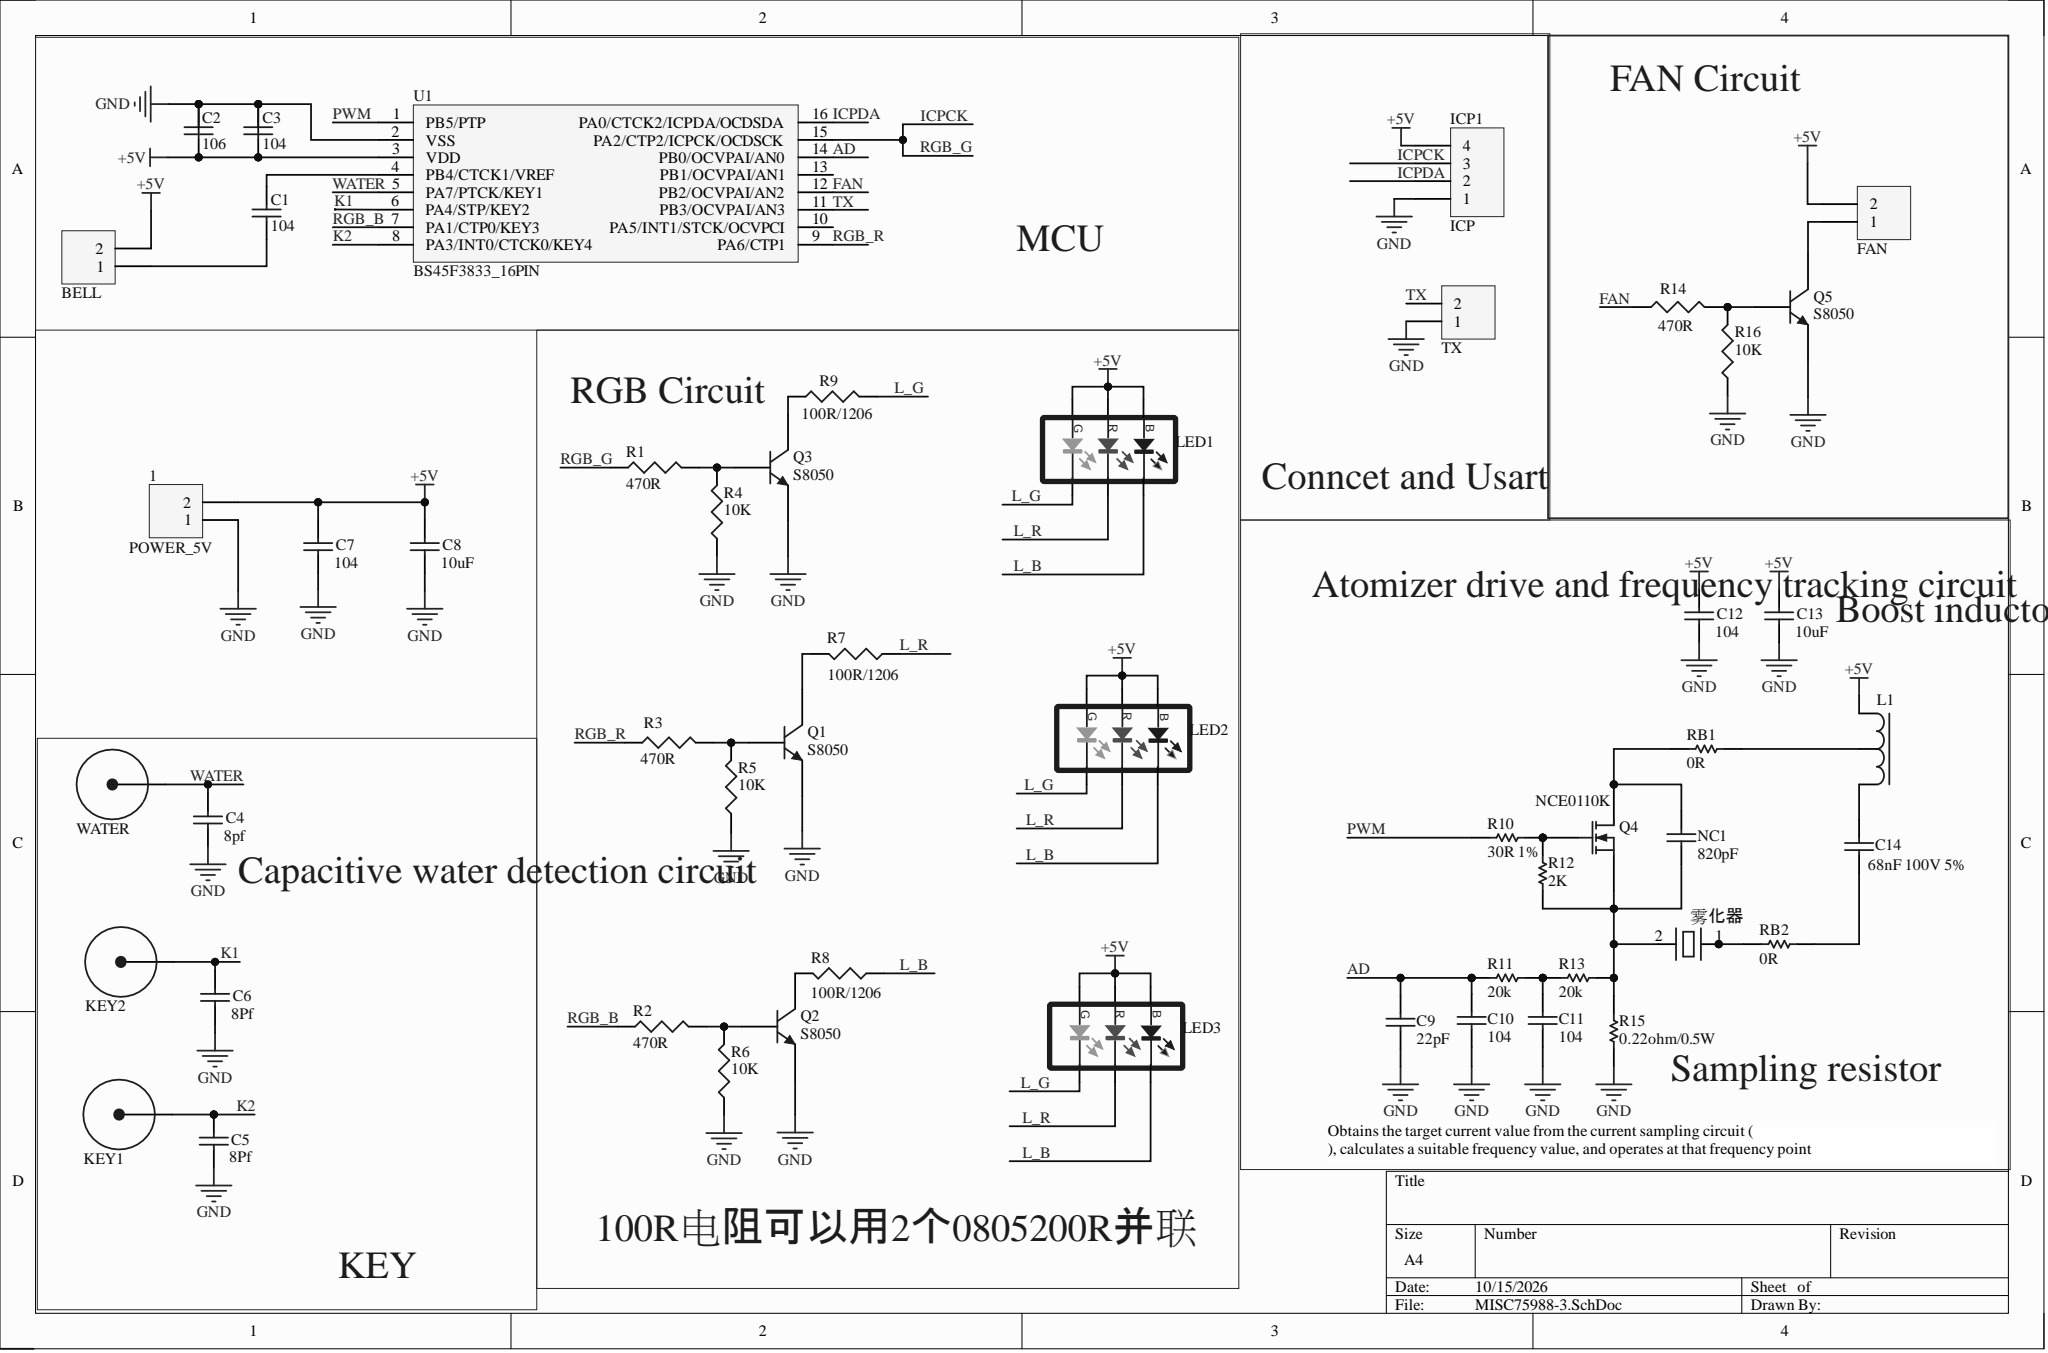Circuit board | Altium Designer | 52 parts | 34 nets
Bill of materials:
Comment,Description,Designator,Footprint,LibRef,Quantity
"POWER_5V","Header, 2-Pin","1","con2-wafer","Header 2","1"
"BELL","Header, 2-Pin","BELL","con2-wafer","Header 2","1"
"0.1uF","Capacitor","C1, C2, C3","0603C","Cap","3"
"CAP","","C4, C5, C6, C7, C8, C10, C11, C12, C13, C14, NC1","0603C","CAP_4","11"
"22pF","","C9","0603C","CAP_4","1"
"FAN","Header, 2-Pin","FAN1","con2-wafer","Header 2","1"
"ICP","Header, 4-Pin","ICP1","HDR1X4","Header 4","1"
"KEY1","","KEY1","TP2","Touch-Pad","1"
"KEY2","","KEY2","TP2","Touch-Pad","1"
"INDUCTOR","","L1","TREE","INDUCTOR5","1"
"RGB","","LED1, LED2, LED3","LED-5050","RGB-CREE(5)","3"
"S8050","NPN General Purpose Amplifier","Q1, Q2, Q3, Q5","SOT_23","2N3904","4"
"NCE0110K","N-Channel MOSFET","Q4","TO252-3","MOSFET-N","1"
"2.2K","Resistor","R1, R2, R4, R5, R6, R16","0603R","Res3","6"
"15R","Resistor","R3","0603R","Res3","1"
"100R/1206","Resistor","R7, R8, R9","0603R","Res3","3"
"RES","","R10, R11, R12, R13, RB1, RB2","0603R","RES_4","6"
"","Resistor","R14","0603R","Res3","1"
"RES","","R15","2512","RES_4","1"
"TX","Header, 2-Pin","TX1","HDR1X2","Header 2","1"
"BS45F3833_16PIN","","U1","NSOP 16","BS45F3833_16PIN","1"
"WATER","","WATER1","Touch-Pad","Touch-Pad","1"
"","","雾化器","con2-wafer","CRYSTAL_1","1"
Netlist (Protel format):
[
1
con2-wafer
POWER_5V



]
[
BELL
con2-wafer
BELL



]
[
C1
0603C
0.1uF



]
[
C2
0603C
0.1uF



]
[
C3
0603C
0.1uF



]
[
C4
0603C
CAP



]
[
C5
0603C
CAP



]
[
C6
0603C
CAP



]
[
C7
0603C
CAP



]
[
C8
0603C
CAP



]
[
C9
0603C
22pF



]
[
C10
0603C
CAP



]
[
C11
0603C
CAP



]
[
C12
0603C
CAP



]
[
C13
0603C
CAP



]
[
C14
0603C
CAP



]
[
FAN1
con2-wafer
FAN



]
[
ICP1
HDR1X4
ICP



]
[
KEY1
TP2
KEY1



]
[
KEY2
TP2
KEY2



]
[
L1
TREE
INDUCTOR



]
[
LED1
LED-5050
RGB



]
[
LED2
LED-5050
RGB



]
[
LED3
LED-5050
RGB



]
[
NC1
0603C
CAP



]
[
Q1
SOT_23
S8050



]
[
Q2
SOT_23
S8050



]
[
Q3
SOT_23
S8050



]
[
Q4
TO252-3
NCE0110K



]
[
Q5
SOT_23
S8050



]
[
R1
0603R
2.2K



]
[
R2
0603R
2.2K



]
[
R3
0603R
15R



]
[
R4
0603R
2.2K



]
[
R5
0603R
2.2K



]
[
R6
0603R
2.2K



]
[
R7
0603R
100R/1206



]
[
R8
0603R
100R/1206



]
[
R9
0603R
100R/1206



]
[
R10
0603R
RES



]
[
R11
0603R
RES



]
[
R12
0603R
RES



]
[
R13
0603R
RES



]
[
R14
0603R




]
[
R15
2512
RES



]
[
R16
0603R
2.2K



]
[
RB1
0603R
RES



]
[
RB2
0603R
RES



]
[
TX1
HDR1X2
TX



]
[
U1
NSOP 16
BS45F3833_16PIN



]
[
WATER1
Touch-Pad
WATER



]
[
雾化器
con2-wafer




]
(
WATER
C4-2
U1-5
WATER1-1
)
(
TX
TX1-2
U1-11
)
(
RGB_R
R3-1
U1-9
)
(
RGB_B
R2-1
U1-7
)
(
PWM
R10-1
U1-1
)
(
NetRB2_1
RB2-1
雾化器-1
)
(
NetQ5_2
Q5-2
R14-2
R16-2
)
(
NetQ4_1
Q4-1
R10-2
R12-2
)
(
NetQ3_3
Q3-3
R9-1
)
(
NetQ3_2
Q3-2
R1-2
R4-2
)
(
NetQ2_3
Q2-3
R8-2
)
(
NetQ2_2
Q2-2
R2-2
R6-2
)
(
NetQ1_3
Q1-3
R7-2
)
(
NetQ1_2
Q1-2
R3-2
R5-2
)
(
NetNC1_2
NC1-2
Q4-2
RB1-1
)
(
NetNC1_1
NC1-1
Q4-3
R12-1
R13-2
R15-2
雾化器-2
)
(
NetL1_2
L1-2
RB1-2
)
(
NetFAN1_1
FAN1-1
Q5-3
)
(
NetC14_2
C14-2
L1-3
)
(
NetC14_1
C14-1
RB2-2
)
(
NetC11_2
C11-2
R11-2
R13-1
)
(
NetC1_2
C1-2
U1-4
)
(
NetBELL_1
BELL-1
C1-1
)
(
L_R
LED1-4
LED2-4
LED3-4
R7-1
)
(
L_G
LED1-5
LED2-5
LED3-5
R9-2
)
(
L_B
LED1-6
LED2-6
LED3-6
R8-1
)
(
K2
C5-2
KEY1-1
U1-8
)
(
K1
C6-2
KEY2-1
U1-6
)
(
ICPDA
ICP1-2
U1-16
)
(
ICPCK
ICP1-3
R1-1
U1-15
)
(
GND
1-1
C2-2
C3-2
C4-1
C5-1
C6-1
C7-1
C8-1
C9-1
C10-1
C11-1
C12-1
C13-1
ICP1-1
Q1-1
Q2-1
Q3-1
Q5-1
R4-1
R5-1
R6-1
R15-1
R16-1
TX1-1
U1-2
)
(
FAN
R14-1
U1-12
)
(
AD
C9-2
C10-2
R11-1
U1-14
)
(
+5V
1-2
BELL-2
C2-1
C3-1
C7-2
C8-2
C12-2
C13-2
FAN1-2
ICP1-4
L1-1
LED1-1
LED1-2
LED1-3
LED2-1
LED2-2
LED2-3
LED3-1
LED3-2
LED3-3
U1-3
)